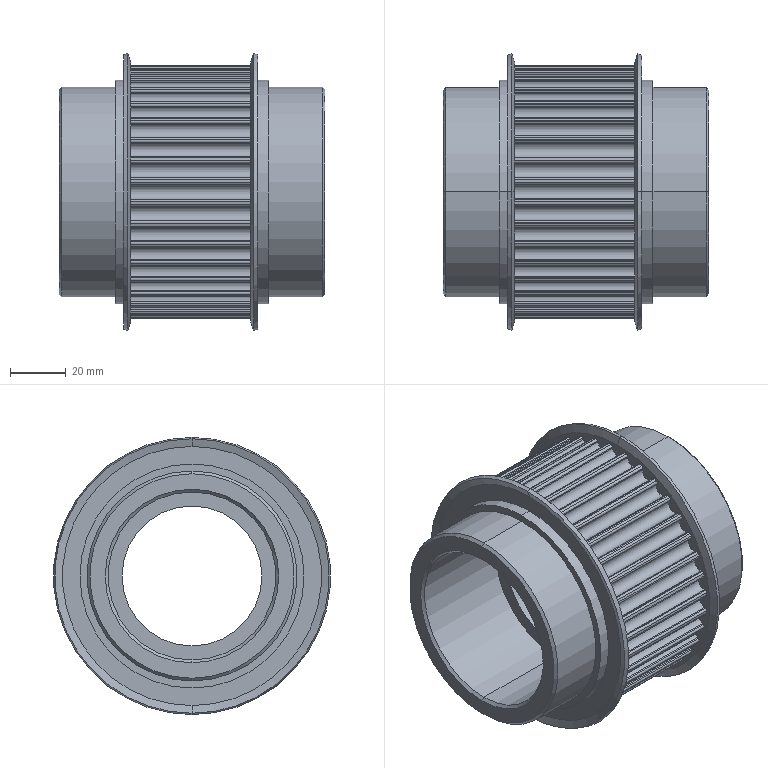Part | SolidWorks | features ICE 8, Chamfer 4, Cut 2, Revolution 2, CirPattern 1, MirrorPattern 1, MirrorSolid 1, RefAxis 1 | 2 solids | 295 faces | box 95 x 99 x 99 mm | volume 277778 mm3 | cylinder 193 | plane 82 | cone 20 | commonest cylinder face diameters 1.56 x90 5.14 x53 90.298 x36 80 x6 75 x4 50 x2